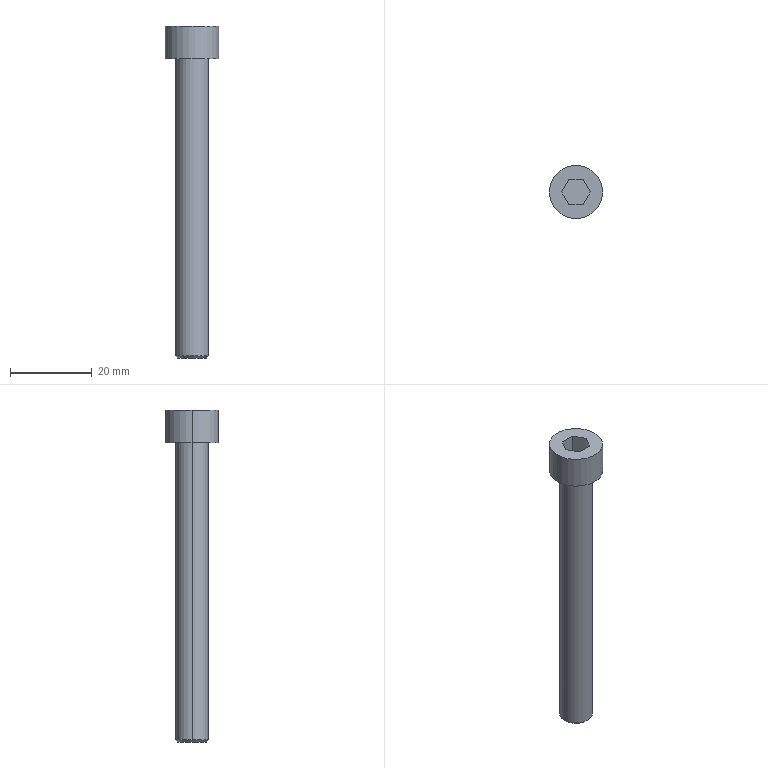Part | Creo | 1 solid | 16 faces | box 13 x 13 x 81 mm | volume 4564 mm3 | plane 10 | cylinder 4 | cone 2 | commonest cylinder face diameters 8 x2 13 x2
STEP:
#1=CARTESIAN_POINT('',(0.,0.,0.));
#2=DIRECTION('',(0.,0.,1.));
#3=DIRECTION('',(1.,0.,0.));
#4=AXIS2_PLACEMENT_3D('',#1,#2,#3);
#5=CARTESIAN_POINT('',(-46.168,197.873,-110.934));
#6=VERTEX_POINT('',#5);
#7=CARTESIAN_POINT('',(-38.168,197.873,-110.934));
#8=VERTEX_POINT('',#7);
#9=CARTESIAN_POINT('',(-42.168,197.873,-110.934));
#10=DIRECTION('',(0.,0.,-1.));
#11=DIRECTION('',(-1.,0.,0.));
#12=AXIS2_PLACEMENT_3D('',#9,#10,#11);
#13=CIRCLE('',#12,4.);
#14=EDGE_CURVE('',#6,#8,#13,.T.);
#15=ORIENTED_EDGE('',*,*,#14,.T.);
#16=CARTESIAN_POINT('',(-38.168,197.873,-38.441));
#17=VERTEX_POINT('',#16);
#18=CARTESIAN_POINT('',(-38.168,197.873,-38.441));
#19=DIRECTION('',(0.,0.,-1.));
#20=VECTOR('',#19,72.493);
#21=LINE('',#18,#20);
#22=EDGE_CURVE('',#17,#8,#21,.T.);
#23=ORIENTED_EDGE('',*,*,#22,.F.);
#24=CARTESIAN_POINT('',(-46.168,197.873,-38.441));
#25=VERTEX_POINT('',#24);
#26=CARTESIAN_POINT('',(-42.168,197.873,-38.441));
#27=DIRECTION('',(0.,0.,1.));
#28=DIRECTION('',(1.,0.,0.));
#29=AXIS2_PLACEMENT_3D('',#26,#27,#28);
#30=CIRCLE('',#29,4.);
#31=EDGE_CURVE('',#17,#25,#30,.T.);
#32=ORIENTED_EDGE('',*,*,#31,.T.);
#33=CARTESIAN_POINT('',(-46.168,197.873,-38.441));
#34=DIRECTION('',(0.,0.,-1.));
#35=VECTOR('',#34,72.493);
#36=LINE('',#33,#35);
#37=EDGE_CURVE('',#25,#6,#36,.T.);
#38=ORIENTED_EDGE('',*,*,#37,.T.);
#39=EDGE_LOOP('',(#15,#23,#32,#38));
#40=FACE_OUTER_BOUND('',#39,.F.);
#41=CARTESIAN_POINT('',(-42.168,197.873,-38.441));
#42=DIRECTION('',(0.,0.,-1.));
#43=DIRECTION('',(-1.,0.,0.));
#44=AXIS2_PLACEMENT_3D('',#41,#42,#43);
#45=CYLINDRICAL_SURFACE('',#44,4.);
#46=ADVANCED_FACE('',(#40),#45,.T.);
#47=CARTESIAN_POINT('',(-45.661,197.873,-111.441));
#48=VERTEX_POINT('',#47);
#49=CARTESIAN_POINT('',(-38.676,197.873,-111.441));
#50=VERTEX_POINT('',#49);
#51=CARTESIAN_POINT('',(-42.168,197.873,-111.441));
#52=DIRECTION('',(0.,0.,-1.));
#53=DIRECTION('',(-1.,0.,0.));
#54=AXIS2_PLACEMENT_3D('',#51,#52,#53);
#55=CIRCLE('',#54,3.493);
#56=EDGE_CURVE('',#48,#50,#55,.T.);
#57=ORIENTED_EDGE('',*,*,#56,.T.);
#58=CARTESIAN_POINT('',(-38.676,197.873,-111.441));
#59=DIRECTION('',(0.7071,0.,0.7071));
#60=VECTOR('',#59,0.7176);
#61=LINE('',#58,#60);
#62=EDGE_CURVE('',#50,#8,#61,.T.);
#63=ORIENTED_EDGE('',*,*,#62,.T.);
#64=ORIENTED_EDGE('',*,*,#14,.F.);
#65=CARTESIAN_POINT('',(-45.661,197.873,-111.441));
#66=DIRECTION('',(-0.7071,0.,0.7071));
#67=VECTOR('',#66,0.7176);
#68=LINE('',#65,#67);
#69=EDGE_CURVE('',#48,#6,#68,.T.);
#70=ORIENTED_EDGE('',*,*,#69,.F.);
#71=EDGE_LOOP('',(#57,#63,#64,#70));
#72=FACE_OUTER_BOUND('',#71,.F.);
#73=CARTESIAN_POINT('',(-42.168,197.873,-111.188));
#74=DIRECTION('',(0.,0.,1.));
#75=DIRECTION('',(1.,0.,0.));
#76=AXIS2_PLACEMENT_3D('',#73,#74,#75);
#77=CONICAL_SURFACE('',#76,3.746,45.);
#78=ADVANCED_FACE('',(#72),#77,.T.);
#79=CARTESIAN_POINT('',(-42.168,197.873,-111.441));
#80=DIRECTION('',(0.,0.,-1.));
#81=DIRECTION('',(1.,0.,0.));
#82=AXIS2_PLACEMENT_3D('',#79,#80,#81);
#83=CIRCLE('',#82,3.493);
#84=EDGE_CURVE('',#50,#48,#83,.T.);
#85=ORIENTED_EDGE('',*,*,#84,.F.);
#86=ORIENTED_EDGE('',*,*,#56,.F.);
#87=EDGE_LOOP('',(#85,#86));
#88=FACE_OUTER_BOUND('',#87,.F.);
#89=CARTESIAN_POINT('',(-42.168,197.873,-111.441));
#90=DIRECTION('',(0.,0.,1.));
#91=DIRECTION('',(1.,0.,0.));
#92=AXIS2_PLACEMENT_3D('',#89,#90,#91);
#93=PLANE('',#92);
#94=ADVANCED_FACE('',(#88),#93,.F.);
#95=ORIENTED_EDGE('',*,*,#84,.T.);
#96=ORIENTED_EDGE('',*,*,#69,.T.);
#97=CARTESIAN_POINT('',(-42.168,197.873,-110.934));
#98=DIRECTION('',(0.,0.,-1.));
#99=DIRECTION('',(1.,0.,0.));
#100=AXIS2_PLACEMENT_3D('',#97,#98,#99);
#101=CIRCLE('',#100,4.);
#102=EDGE_CURVE('',#8,#6,#101,.T.);
#103=ORIENTED_EDGE('',*,*,#102,.F.);
#104=ORIENTED_EDGE('',*,*,#62,.F.);
#105=EDGE_LOOP('',(#95,#96,#103,#104));
#106=FACE_OUTER_BOUND('',#105,.F.);
#107=CARTESIAN_POINT('',(-42.168,197.873,-111.188));
#108=DIRECTION('',(0.,0.,1.));
#109=DIRECTION('',(1.,0.,0.));
#110=AXIS2_PLACEMENT_3D('',#107,#108,#109);
#111=CONICAL_SURFACE('',#110,3.746,45.);
#112=ADVANCED_FACE('',(#106),#111,.T.);
#113=ORIENTED_EDGE('',*,*,#102,.T.);
#114=ORIENTED_EDGE('',*,*,#37,.F.);
#115=CARTESIAN_POINT('',(-42.168,197.873,-38.441));
#116=DIRECTION('',(0.,0.,1.));
#117=DIRECTION('',(-1.,0.,0.));
#118=AXIS2_PLACEMENT_3D('',#115,#116,#117);
#119=CIRCLE('',#118,4.);
#120=EDGE_CURVE('',#25,#17,#119,.T.);
#121=ORIENTED_EDGE('',*,*,#120,.T.);
#122=ORIENTED_EDGE('',*,*,#22,.T.);
#123=EDGE_LOOP('',(#113,#114,#121,#122));
#124=FACE_OUTER_BOUND('',#123,.F.);
#125=CARTESIAN_POINT('',(-42.168,197.873,-38.441));
#126=DIRECTION('',(0.,0.,-1.));
#127=DIRECTION('',(-1.,0.,0.));
#128=AXIS2_PLACEMENT_3D('',#125,#126,#127);
#129=CYLINDRICAL_SURFACE('',#128,4.);
#130=ADVANCED_FACE('',(#124),#129,.T.);
#131=CARTESIAN_POINT('',(-35.668,197.873,-38.441));
#132=VERTEX_POINT('',#131);
#133=CARTESIAN_POINT('',(-48.668,197.873,-38.441));
#134=VERTEX_POINT('',#133);
#135=CARTESIAN_POINT('',(-42.168,197.873,-38.441));
#136=DIRECTION('',(0.,0.,-1.));
#137=DIRECTION('',(1.,0.,0.));
#138=AXIS2_PLACEMENT_3D('',#135,#136,#137);
#139=CIRCLE('',#138,6.5);
#140=EDGE_CURVE('',#132,#134,#139,.T.);
#141=ORIENTED_EDGE('',*,*,#140,.F.);
#142=CARTESIAN_POINT('',(-42.168,197.873,-38.441));
#143=DIRECTION('',(0.,0.,-1.));
#144=DIRECTION('',(-1.,0.,0.));
#145=AXIS2_PLACEMENT_3D('',#142,#143,#144);
#146=CIRCLE('',#145,6.5);
#147=EDGE_CURVE('',#134,#132,#146,.T.);
#148=ORIENTED_EDGE('',*,*,#147,.F.);
#149=EDGE_LOOP('',(#141,#148));
#150=FACE_OUTER_BOUND('',#149,.F.);
#151=ORIENTED_EDGE('',*,*,#31,.F.);
#152=ORIENTED_EDGE('',*,*,#120,.F.);
#153=EDGE_LOOP('',(#151,#152));
#154=FACE_BOUND('',#153,.F.);
#155=CARTESIAN_POINT('',(-42.168,197.873,-38.441));
#156=DIRECTION('',(0.,0.,-1.));
#157=DIRECTION('',(-1.,0.,0.));
#158=AXIS2_PLACEMENT_3D('',#155,#156,#157);
#159=PLANE('',#158);
#160=ADVANCED_FACE('',(#150,#154),#159,.T.);
#161=CARTESIAN_POINT('',(-48.668,197.873,-30.441));
#162=VERTEX_POINT('',#161);
#163=CARTESIAN_POINT('',(-35.668,197.873,-30.441));
#164=VERTEX_POINT('',#163);
#165=CARTESIAN_POINT('',(-42.168,197.873,-30.441));
#166=DIRECTION('',(0.,0.,1.));
#167=DIRECTION('',(-1.,0.,0.));
#168=AXIS2_PLACEMENT_3D('',#165,#166,#167);
#169=CIRCLE('',#168,6.5);
#170=EDGE_CURVE('',#162,#164,#169,.T.);
#171=ORIENTED_EDGE('',*,*,#170,.T.);
#172=CARTESIAN_POINT('',(-35.668,197.873,-38.441));
#173=DIRECTION('',(0.,0.,1.));
#174=VECTOR('',#173,8.);
#175=LINE('',#172,#174);
#176=EDGE_CURVE('',#132,#164,#175,.T.);
#177=ORIENTED_EDGE('',*,*,#176,.F.);
#178=ORIENTED_EDGE('',*,*,#140,.T.);
#179=CARTESIAN_POINT('',(-48.668,197.873,-38.441));
#180=DIRECTION('',(0.,0.,1.));
#181=VECTOR('',#180,8.);
#182=LINE('',#179,#181);
#183=EDGE_CURVE('',#134,#162,#182,.T.);
#184=ORIENTED_EDGE('',*,*,#183,.T.);
#185=EDGE_LOOP('',(#171,#177,#178,#184));
#186=FACE_OUTER_BOUND('',#185,.F.);
#187=CARTESIAN_POINT('',(-42.168,197.873,-38.441));
#188=DIRECTION('',(0.,0.,1.));
#189=DIRECTION('',(1.,0.,0.));
#190=AXIS2_PLACEMENT_3D('',#187,#188,#189);
#191=CYLINDRICAL_SURFACE('',#190,6.5);
#192=ADVANCED_FACE('',(#186),#191,.T.);
#193=CARTESIAN_POINT('',(-42.168,197.873,-30.441));
#194=DIRECTION('',(0.,0.,1.));
#195=DIRECTION('',(1.,0.,0.));
#196=AXIS2_PLACEMENT_3D('',#193,#194,#195);
#197=CIRCLE('',#196,6.5);
#198=EDGE_CURVE('',#164,#162,#197,.T.);
#199=ORIENTED_EDGE('',*,*,#198,.F.);
#200=ORIENTED_EDGE('',*,*,#170,.F.);
#201=EDGE_LOOP('',(#199,#200));
#202=FACE_OUTER_BOUND('',#201,.F.);
#203=CARTESIAN_POINT('',(-40.436,194.873,-30.441));
#204=VERTEX_POINT('',#203);
#205=CARTESIAN_POINT('',(-43.9,194.873,-30.441));
#206=VERTEX_POINT('',#205);
#207=CARTESIAN_POINT('',(-40.436,194.873,-30.441));
#208=DIRECTION('',(-1.,0.,0.));
#209=VECTOR('',#208,3.464);
#210=LINE('',#207,#209);
#211=EDGE_CURVE('',#204,#206,#210,.T.);
#212=ORIENTED_EDGE('',*,*,#211,.F.);
#213=CARTESIAN_POINT('',(-38.704,197.873,-30.441));
#214=VERTEX_POINT('',#213);
#215=CARTESIAN_POINT('',(-38.704,197.873,-30.441));
#216=DIRECTION('',(-0.5,-0.866,0.));
#217=VECTOR('',#216,3.464);
#218=LINE('',#215,#217);
#219=EDGE_CURVE('',#214,#204,#218,.T.);
#220=ORIENTED_EDGE('',*,*,#219,.F.);
#221=CARTESIAN_POINT('',(-40.436,200.873,-30.441));
#222=VERTEX_POINT('',#221);
#223=CARTESIAN_POINT('',(-40.436,200.873,-30.441));
#224=DIRECTION('',(0.5,-0.866,0.));
#225=VECTOR('',#224,3.464);
#226=LINE('',#223,#225);
#227=EDGE_CURVE('',#222,#214,#226,.T.);
#228=ORIENTED_EDGE('',*,*,#227,.F.);
#229=CARTESIAN_POINT('',(-43.9,200.873,-30.441));
#230=VERTEX_POINT('',#229);
#231=CARTESIAN_POINT('',(-43.9,200.873,-30.441));
#232=DIRECTION('',(1.,0.,0.));
#233=VECTOR('',#232,3.464);
#234=LINE('',#231,#233);
#235=EDGE_CURVE('',#230,#222,#234,.T.);
#236=ORIENTED_EDGE('',*,*,#235,.F.);
#237=CARTESIAN_POINT('',(-45.632,197.873,-30.441));
#238=VERTEX_POINT('',#237);
#239=CARTESIAN_POINT('',(-45.632,197.873,-30.441));
#240=DIRECTION('',(0.5,0.866,0.));
#241=VECTOR('',#240,3.464);
#242=LINE('',#239,#241);
#243=EDGE_CURVE('',#238,#230,#242,.T.);
#244=ORIENTED_EDGE('',*,*,#243,.F.);
#245=CARTESIAN_POINT('',(-43.9,194.873,-30.441));
#246=DIRECTION('',(-0.5,0.866,0.));
#247=VECTOR('',#246,3.464);
#248=LINE('',#245,#247);
#249=EDGE_CURVE('',#206,#238,#248,.T.);
#250=ORIENTED_EDGE('',*,*,#249,.F.);
#251=EDGE_LOOP('',(#212,#220,#228,#236,#244,#250));
#252=FACE_BOUND('',#251,.F.);
#253=CARTESIAN_POINT('',(-42.168,197.873,-30.441));
#254=DIRECTION('',(0.,0.,1.));
#255=DIRECTION('',(1.,0.,0.));
#256=AXIS2_PLACEMENT_3D('',#253,#254,#255);
#257=PLANE('',#256);
#258=ADVANCED_FACE('',(#202,#252),#257,.T.);
#259=ORIENTED_EDGE('',*,*,#211,.T.);
#260=CARTESIAN_POINT('',(-43.9,194.873,-35.721));
#261=VERTEX_POINT('',#260);
#262=CARTESIAN_POINT('',(-43.9,194.873,-30.441));
#263=DIRECTION('',(0.,0.,-1.));
#264=VECTOR('',#263,5.28);
#265=LINE('',#262,#264);
#266=EDGE_CURVE('',#206,#261,#265,.T.);
#267=ORIENTED_EDGE('',*,*,#266,.T.);
#268=CARTESIAN_POINT('',(-40.436,194.873,-35.721));
#269=VERTEX_POINT('',#268);
#270=CARTESIAN_POINT('',(-40.436,194.873,-35.721));
#271=DIRECTION('',(-1.,0.,0.));
#272=VECTOR('',#271,3.464);
#273=LINE('',#270,#272);
#274=EDGE_CURVE('',#269,#261,#273,.T.);
#275=ORIENTED_EDGE('',*,*,#274,.F.);
#276=CARTESIAN_POINT('',(-40.436,194.873,-30.441));
#277=DIRECTION('',(0.,0.,-1.));
#278=VECTOR('',#277,5.28);
#279=LINE('',#276,#278);
#280=EDGE_CURVE('',#204,#269,#279,.T.);
#281=ORIENTED_EDGE('',*,*,#280,.F.);
#282=EDGE_LOOP('',(#259,#267,#275,#281));
#283=FACE_OUTER_BOUND('',#282,.F.);
#284=CARTESIAN_POINT('',(-43.9,194.873,-35.721));
#285=DIRECTION('',(0.,-1.,0.));
#286=DIRECTION('',(0.,0.,-1.));
#287=AXIS2_PLACEMENT_3D('',#284,#285,#286);
#288=PLANE('',#287);
#289=ADVANCED_FACE('',(#283),#288,.F.);
#290=ORIENTED_EDGE('',*,*,#249,.T.);
#291=CARTESIAN_POINT('',(-45.632,197.873,-35.721));
#292=VERTEX_POINT('',#291);
#293=CARTESIAN_POINT('',(-45.632,197.873,-30.441));
#294=DIRECTION('',(0.,0.,-1.));
#295=VECTOR('',#294,5.28);
#296=LINE('',#293,#295);
#297=EDGE_CURVE('',#238,#292,#296,.T.);
#298=ORIENTED_EDGE('',*,*,#297,.T.);
#299=CARTESIAN_POINT('',(-45.632,197.873,-35.721));
#300=DIRECTION('',(0.5,-0.866,0.));
#301=VECTOR('',#300,3.464);
#302=LINE('',#299,#301);
#303=EDGE_CURVE('',#292,#261,#302,.T.);
#304=ORIENTED_EDGE('',*,*,#303,.T.);
#305=ORIENTED_EDGE('',*,*,#266,.F.);
#306=EDGE_LOOP('',(#290,#298,#304,#305));
#307=FACE_OUTER_BOUND('',#306,.F.);
#308=CARTESIAN_POINT('',(-45.632,197.873,-35.721));
#309=DIRECTION('',(-0.866,-0.5,0.));
#310=DIRECTION('',(0.5,-0.866,0.));
#311=AXIS2_PLACEMENT_3D('',#308,#309,#310);
#312=PLANE('',#311);
#313=ADVANCED_FACE('',(#307),#312,.F.);
#314=ORIENTED_EDGE('',*,*,#243,.T.);
#315=CARTESIAN_POINT('',(-43.9,200.873,-35.721));
#316=VERTEX_POINT('',#315);
#317=CARTESIAN_POINT('',(-43.9,200.873,-30.441));
#318=DIRECTION('',(0.,0.,-1.));
#319=VECTOR('',#318,5.28);
#320=LINE('',#317,#319);
#321=EDGE_CURVE('',#230,#316,#320,.T.);
#322=ORIENTED_EDGE('',*,*,#321,.T.);
#323=CARTESIAN_POINT('',(-43.9,200.873,-35.721));
#324=DIRECTION('',(-0.5,-0.866,0.));
#325=VECTOR('',#324,3.464);
#326=LINE('',#323,#325);
#327=EDGE_CURVE('',#316,#292,#326,.T.);
#328=ORIENTED_EDGE('',*,*,#327,.T.);
#329=ORIENTED_EDGE('',*,*,#297,.F.);
#330=EDGE_LOOP('',(#314,#322,#328,#329));
#331=FACE_OUTER_BOUND('',#330,.F.);
#332=CARTESIAN_POINT('',(-43.9,200.873,-35.721));
#333=DIRECTION('',(-0.866,0.5,0.));
#334=DIRECTION('',(-0.5,-0.866,0.));
#335=AXIS2_PLACEMENT_3D('',#332,#333,#334);
#336=PLANE('',#335);
#337=ADVANCED_FACE('',(#331),#336,.F.);
#338=ORIENTED_EDGE('',*,*,#235,.T.);
#339=CARTESIAN_POINT('',(-40.436,200.873,-35.721));
#340=VERTEX_POINT('',#339);
#341=CARTESIAN_POINT('',(-40.436,200.873,-30.441));
#342=DIRECTION('',(0.,0.,-1.));
#343=VECTOR('',#342,5.28);
#344=LINE('',#341,#343);
#345=EDGE_CURVE('',#222,#340,#344,.T.);
#346=ORIENTED_EDGE('',*,*,#345,.T.);
#347=CARTESIAN_POINT('',(-43.9,200.873,-35.721));
#348=DIRECTION('',(1.,0.,0.));
#349=VECTOR('',#348,3.464);
#350=LINE('',#347,#349);
#351=EDGE_CURVE('',#316,#340,#350,.T.);
#352=ORIENTED_EDGE('',*,*,#351,.F.);
#353=ORIENTED_EDGE('',*,*,#321,.F.);
#354=EDGE_LOOP('',(#338,#346,#352,#353));
#355=FACE_OUTER_BOUND('',#354,.F.);
#356=CARTESIAN_POINT('',(-40.436,200.873,-35.721));
#357=DIRECTION('',(0.,1.,0.));
#358=DIRECTION('',(0.,0.,1.));
#359=AXIS2_PLACEMENT_3D('',#356,#357,#358);
#360=PLANE('',#359);
#361=ADVANCED_FACE('',(#355),#360,.F.);
#362=ORIENTED_EDGE('',*,*,#227,.T.);
#363=CARTESIAN_POINT('',(-38.704,197.873,-35.721));
#364=VERTEX_POINT('',#363);
#365=CARTESIAN_POINT('',(-38.704,197.873,-30.441));
#366=DIRECTION('',(0.,0.,-1.));
#367=VECTOR('',#366,5.28);
#368=LINE('',#365,#367);
#369=EDGE_CURVE('',#214,#364,#368,.T.);
#370=ORIENTED_EDGE('',*,*,#369,.T.);
#371=CARTESIAN_POINT('',(-38.704,197.873,-35.721));
#372=DIRECTION('',(-0.5,0.866,0.));
#373=VECTOR('',#372,3.464);
#374=LINE('',#371,#373);
#375=EDGE_CURVE('',#364,#340,#374,.T.);
#376=ORIENTED_EDGE('',*,*,#375,.T.);
#377=ORIENTED_EDGE('',*,*,#345,.F.);
#378=EDGE_LOOP('',(#362,#370,#376,#377));
#379=FACE_OUTER_BOUND('',#378,.F.);
#380=CARTESIAN_POINT('',(-38.704,197.873,-35.721));
#381=DIRECTION('',(0.866,0.5,0.));
#382=DIRECTION('',(-0.5,0.866,0.));
#383=AXIS2_PLACEMENT_3D('',#380,#381,#382);
#384=PLANE('',#383);
#385=ADVANCED_FACE('',(#379),#384,.F.);
#386=ORIENTED_EDGE('',*,*,#219,.T.);
#387=ORIENTED_EDGE('',*,*,#280,.T.);
#388=CARTESIAN_POINT('',(-40.436,194.873,-35.721));
#389=DIRECTION('',(0.5,0.866,0.));
#390=VECTOR('',#389,3.464);
#391=LINE('',#388,#390);
#392=EDGE_CURVE('',#269,#364,#391,.T.);
#393=ORIENTED_EDGE('',*,*,#392,.T.);
#394=ORIENTED_EDGE('',*,*,#369,.F.);
#395=EDGE_LOOP('',(#386,#387,#393,#394));
#396=FACE_OUTER_BOUND('',#395,.F.);
#397=CARTESIAN_POINT('',(-40.436,194.873,-35.721));
#398=DIRECTION('',(0.866,-0.5,0.));
#399=DIRECTION('',(0.5,0.866,0.));
#400=AXIS2_PLACEMENT_3D('',#397,#398,#399);
#401=PLANE('',#400);
#402=ADVANCED_FACE('',(#396),#401,.F.);
#403=ORIENTED_EDGE('',*,*,#274,.T.);
#404=ORIENTED_EDGE('',*,*,#303,.F.);
#405=ORIENTED_EDGE('',*,*,#327,.F.);
#406=ORIENTED_EDGE('',*,*,#351,.T.);
#407=ORIENTED_EDGE('',*,*,#375,.F.);
#408=ORIENTED_EDGE('',*,*,#392,.F.);
#409=EDGE_LOOP('',(#403,#404,#405,#406,#407,#408));
#410=FACE_OUTER_BOUND('',#409,.F.);
#411=CARTESIAN_POINT('',(-40.436,194.873,-35.721));
#412=DIRECTION('',(0.,0.,1.));
#413=DIRECTION('',(1.,0.,0.));
#414=AXIS2_PLACEMENT_3D('',#411,#412,#413);
#415=PLANE('',#414);
#416=ADVANCED_FACE('',(#410),#415,.T.);
#417=ORIENTED_EDGE('',*,*,#198,.T.);
#418=ORIENTED_EDGE('',*,*,#183,.F.);
#419=ORIENTED_EDGE('',*,*,#147,.T.);
#420=ORIENTED_EDGE('',*,*,#176,.T.);
#421=EDGE_LOOP('',(#417,#418,#419,#420));
#422=FACE_OUTER_BOUND('',#421,.F.);
#423=CARTESIAN_POINT('',(-42.168,197.873,-38.441));
#424=DIRECTION('',(0.,0.,1.));
#425=DIRECTION('',(1.,0.,0.));
#426=AXIS2_PLACEMENT_3D('',#423,#424,#425);
#427=CYLINDRICAL_SURFACE('',#426,6.5);
#428=ADVANCED_FACE('',(#422),#427,.T.);
#429=CLOSED_SHELL('',(#46,#78,#94,#112,#130,#160,#192,#258,#289,#313,#337,#361,#385,#402,#416,#428));
#430=MANIFOLD_SOLID_BREP('',#429);
#431=(LENGTH_UNIT()NAMED_UNIT(*)SI_UNIT(.MILLI.,.METRE.));
#432=UNCERTAINTY_MEASURE_WITH_UNIT(LENGTH_MEASURE(0.008306),#431,'','');
#433=(NAMED_UNIT(*)PLANE_ANGLE_UNIT()SI_UNIT($,.RADIAN.));
#434=PLANE_ANGLE_MEASURE_WITH_UNIT(PLANE_ANGLE_MEASURE(0.01745),#433);
#435=(CONVERSION_BASED_UNIT('DEGREE',#434)NAMED_UNIT(*)PLANE_ANGLE_UNIT());
#436=(NAMED_UNIT(*)SI_UNIT($,.STERADIAN.)SOLID_ANGLE_UNIT());
#437=(GEOMETRIC_REPRESENTATION_CONTEXT(3)GLOBAL_UNCERTAINTY_ASSIGNED_CONTEXT((#432))GLOBAL_UNIT_ASSIGNED_CONTEXT((#431,#435,#436))REPRESENTATION_CONTEXT('',''));
#438=ADVANCED_BREP_SHAPE_REPRESENTATION('',(#4,#430),#437);